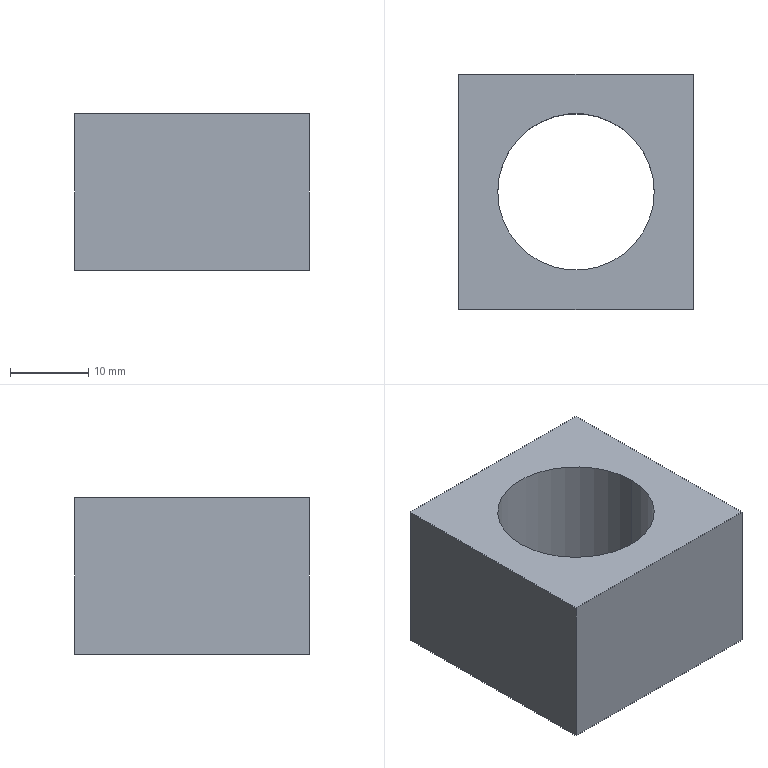Part | SolidWorks | features Extrusion 1 | 1 solid | 8 faces | box 30 x 30 x 20 mm | volume 11717 mm3 | plane 6 | cylinder 2 | commonest cylinder face diameters 20 x2
STEP:
#1=CARTESIAN_POINT('',(-10.,0.,-10.));
#2=VERTEX_POINT('',#1);
#3=CARTESIAN_POINT('',(10.,0.,-10.));
#4=VERTEX_POINT('',#3);
#5=CARTESIAN_POINT('',(0.,0.,-10.));
#6=DIRECTION('',(0.,0.,1.));
#7=DIRECTION('',(-1.,0.,0.));
#8=AXIS2_PLACEMENT_3D('',#5,#6,#7);
#9=CIRCLE('',#8,10.);
#10=EDGE_CURVE('',#2,#4,#9,.T.);
#11=ORIENTED_EDGE('',*,*,#10,.F.);
#12=CARTESIAN_POINT('',(-10.,0.,10.));
#13=VERTEX_POINT('',#12);
#14=CARTESIAN_POINT('',(-10.,0.,-10.));
#15=DIRECTION('',(0.,0.,1.));
#16=VECTOR('',#15,1000.);
#17=LINE('',#14,#16);
#18=EDGE_CURVE('',#2,#13,#17,.T.);
#19=ORIENTED_EDGE('',*,*,#18,.T.);
#20=CARTESIAN_POINT('',(10.,0.,10.));
#21=VERTEX_POINT('',#20);
#22=CARTESIAN_POINT('',(0.,0.,10.));
#23=DIRECTION('',(0.,0.,1.));
#24=DIRECTION('',(-1.,0.,0.));
#25=AXIS2_PLACEMENT_3D('',#22,#23,#24);
#26=CIRCLE('',#25,10.);
#27=EDGE_CURVE('',#13,#21,#26,.T.);
#28=ORIENTED_EDGE('',*,*,#27,.T.);
#29=CARTESIAN_POINT('',(10.,0.,-10.));
#30=DIRECTION('',(0.,0.,1.));
#31=VECTOR('',#30,1000.);
#32=LINE('',#29,#31);
#33=EDGE_CURVE('',#4,#21,#32,.T.);
#34=ORIENTED_EDGE('',*,*,#33,.F.);
#35=EDGE_LOOP('',(#11,#19,#28,#34));
#36=FACE_OUTER_BOUND('',#35,.T.);
#37=CARTESIAN_POINT('',(0.,0.,-10.));
#38=DIRECTION('',(0.,0.,1.));
#39=DIRECTION('',(1.,0.,0.));
#40=AXIS2_PLACEMENT_3D('',#37,#38,#39);
#41=CYLINDRICAL_SURFACE('',#40,10.);
#42=ADVANCED_FACE('',(#36),#41,.F.);
#43=CARTESIAN_POINT('',(-15.,15.,10.));
#44=VERTEX_POINT('',#43);
#45=CARTESIAN_POINT('',(-15.,-15.,10.));
#46=VERTEX_POINT('',#45);
#47=CARTESIAN_POINT('',(-15.,15.,10.));
#48=DIRECTION('',(0.,-1.,0.));
#49=VECTOR('',#48,1000.);
#50=LINE('',#47,#49);
#51=EDGE_CURVE('',#44,#46,#50,.T.);
#52=ORIENTED_EDGE('',*,*,#51,.F.);
#53=CARTESIAN_POINT('',(-15.,15.,-10.));
#54=VERTEX_POINT('',#53);
#55=CARTESIAN_POINT('',(-15.,15.,-10.));
#56=DIRECTION('',(0.,0.,1.));
#57=VECTOR('',#56,1000.);
#58=LINE('',#55,#57);
#59=EDGE_CURVE('',#54,#44,#58,.T.);
#60=ORIENTED_EDGE('',*,*,#59,.F.);
#61=CARTESIAN_POINT('',(-15.,-15.,-10.));
#62=VERTEX_POINT('',#61);
#63=CARTESIAN_POINT('',(-15.,15.,-10.));
#64=DIRECTION('',(0.,-1.,0.));
#65=VECTOR('',#64,1000.);
#66=LINE('',#63,#65);
#67=EDGE_CURVE('',#54,#62,#66,.T.);
#68=ORIENTED_EDGE('',*,*,#67,.T.);
#69=CARTESIAN_POINT('',(-15.,-15.,-10.));
#70=DIRECTION('',(0.,0.,1.));
#71=VECTOR('',#70,1000.);
#72=LINE('',#69,#71);
#73=EDGE_CURVE('',#62,#46,#72,.T.);
#74=ORIENTED_EDGE('',*,*,#73,.T.);
#75=EDGE_LOOP('',(#52,#60,#68,#74));
#76=FACE_OUTER_BOUND('',#75,.T.);
#77=CARTESIAN_POINT('',(-15.,15.,-10.));
#78=DIRECTION('',(-1.,0.,0.));
#79=DIRECTION('',(0.,0.,1.));
#80=AXIS2_PLACEMENT_3D('',#77,#78,#79);
#81=PLANE('',#80);
#82=ADVANCED_FACE('',(#76),#81,.T.);
#83=CARTESIAN_POINT('',(15.,15.,10.));
#84=VERTEX_POINT('',#83);
#85=CARTESIAN_POINT('',(15.,15.,10.));
#86=DIRECTION('',(-1.,0.,0.));
#87=VECTOR('',#86,1000.);
#88=LINE('',#85,#87);
#89=EDGE_CURVE('',#84,#44,#88,.T.);
#90=ORIENTED_EDGE('',*,*,#89,.F.);
#91=CARTESIAN_POINT('',(15.,15.,-10.));
#92=VERTEX_POINT('',#91);
#93=CARTESIAN_POINT('',(15.,15.,-10.));
#94=DIRECTION('',(0.,0.,1.));
#95=VECTOR('',#94,1000.);
#96=LINE('',#93,#95);
#97=EDGE_CURVE('',#92,#84,#96,.T.);
#98=ORIENTED_EDGE('',*,*,#97,.F.);
#99=CARTESIAN_POINT('',(15.,15.,-10.));
#100=DIRECTION('',(-1.,0.,0.));
#101=VECTOR('',#100,1000.);
#102=LINE('',#99,#101);
#103=EDGE_CURVE('',#92,#54,#102,.T.);
#104=ORIENTED_EDGE('',*,*,#103,.T.);
#105=ORIENTED_EDGE('',*,*,#59,.T.);
#106=EDGE_LOOP('',(#90,#98,#104,#105));
#107=FACE_OUTER_BOUND('',#106,.T.);
#108=CARTESIAN_POINT('',(15.,15.,-10.));
#109=DIRECTION('',(0.,1.,0.));
#110=DIRECTION('',(0.,0.,1.));
#111=AXIS2_PLACEMENT_3D('',#108,#109,#110);
#112=PLANE('',#111);
#113=ADVANCED_FACE('',(#107),#112,.T.);
#114=CARTESIAN_POINT('',(15.,-15.,10.));
#115=VERTEX_POINT('',#114);
#116=CARTESIAN_POINT('',(15.,-15.,10.));
#117=DIRECTION('',(0.,1.,0.));
#118=VECTOR('',#117,1000.);
#119=LINE('',#116,#118);
#120=EDGE_CURVE('',#115,#84,#119,.T.);
#121=ORIENTED_EDGE('',*,*,#120,.F.);
#122=CARTESIAN_POINT('',(15.,-15.,-10.));
#123=VERTEX_POINT('',#122);
#124=CARTESIAN_POINT('',(15.,-15.,-10.));
#125=DIRECTION('',(0.,0.,1.));
#126=VECTOR('',#125,1000.);
#127=LINE('',#124,#126);
#128=EDGE_CURVE('',#123,#115,#127,.T.);
#129=ORIENTED_EDGE('',*,*,#128,.F.);
#130=CARTESIAN_POINT('',(15.,-15.,-10.));
#131=DIRECTION('',(0.,1.,0.));
#132=VECTOR('',#131,1000.);
#133=LINE('',#130,#132);
#134=EDGE_CURVE('',#123,#92,#133,.T.);
#135=ORIENTED_EDGE('',*,*,#134,.T.);
#136=ORIENTED_EDGE('',*,*,#97,.T.);
#137=EDGE_LOOP('',(#121,#129,#135,#136));
#138=FACE_OUTER_BOUND('',#137,.T.);
#139=CARTESIAN_POINT('',(15.,-15.,-10.));
#140=DIRECTION('',(1.,0.,0.));
#141=DIRECTION('',(0.,0.,-1.));
#142=AXIS2_PLACEMENT_3D('',#139,#140,#141);
#143=PLANE('',#142);
#144=ADVANCED_FACE('',(#138),#143,.T.);
#145=CARTESIAN_POINT('',(-15.,-15.,10.));
#146=DIRECTION('',(1.,0.,0.));
#147=VECTOR('',#146,1000.);
#148=LINE('',#145,#147);
#149=EDGE_CURVE('',#46,#115,#148,.T.);
#150=ORIENTED_EDGE('',*,*,#149,.F.);
#151=ORIENTED_EDGE('',*,*,#73,.F.);
#152=CARTESIAN_POINT('',(-15.,-15.,-10.));
#153=DIRECTION('',(1.,0.,0.));
#154=VECTOR('',#153,1000.);
#155=LINE('',#152,#154);
#156=EDGE_CURVE('',#62,#123,#155,.T.);
#157=ORIENTED_EDGE('',*,*,#156,.T.);
#158=ORIENTED_EDGE('',*,*,#128,.T.);
#159=EDGE_LOOP('',(#150,#151,#157,#158));
#160=FACE_OUTER_BOUND('',#159,.T.);
#161=CARTESIAN_POINT('',(-15.,-15.,-10.));
#162=DIRECTION('',(0.,-1.,0.));
#163=DIRECTION('',(0.,0.,-1.));
#164=AXIS2_PLACEMENT_3D('',#161,#162,#163);
#165=PLANE('',#164);
#166=ADVANCED_FACE('',(#160),#165,.T.);
#167=CARTESIAN_POINT('',(0.,0.,-10.));
#168=DIRECTION('',(0.,0.,1.));
#169=DIRECTION('',(-1.,0.,0.));
#170=AXIS2_PLACEMENT_3D('',#167,#168,#169);
#171=CIRCLE('',#170,10.);
#172=EDGE_CURVE('',#4,#2,#171,.T.);
#173=ORIENTED_EDGE('',*,*,#172,.T.);
#174=ORIENTED_EDGE('',*,*,#10,.T.);
#175=EDGE_LOOP('',(#173,#174));
#176=FACE_BOUND('',#175,.T.);
#177=ORIENTED_EDGE('',*,*,#67,.F.);
#178=ORIENTED_EDGE('',*,*,#103,.F.);
#179=ORIENTED_EDGE('',*,*,#134,.F.);
#180=ORIENTED_EDGE('',*,*,#156,.F.);
#181=EDGE_LOOP('',(#177,#178,#179,#180));
#182=FACE_OUTER_BOUND('',#181,.T.);
#183=CARTESIAN_POINT('',(0.,0.,-10.));
#184=DIRECTION('',(0.,0.,1.));
#185=DIRECTION('',(1.,0.,0.));
#186=AXIS2_PLACEMENT_3D('',#183,#184,#185);
#187=PLANE('',#186);
#188=ADVANCED_FACE('',(#176,#182),#187,.F.);
#189=CARTESIAN_POINT('',(0.,0.,10.));
#190=DIRECTION('',(0.,0.,1.));
#191=DIRECTION('',(-1.,0.,0.));
#192=AXIS2_PLACEMENT_3D('',#189,#190,#191);
#193=CIRCLE('',#192,10.);
#194=EDGE_CURVE('',#21,#13,#193,.T.);
#195=ORIENTED_EDGE('',*,*,#194,.F.);
#196=ORIENTED_EDGE('',*,*,#27,.F.);
#197=EDGE_LOOP('',(#195,#196));
#198=FACE_BOUND('',#197,.T.);
#199=ORIENTED_EDGE('',*,*,#51,.T.);
#200=ORIENTED_EDGE('',*,*,#149,.T.);
#201=ORIENTED_EDGE('',*,*,#120,.T.);
#202=ORIENTED_EDGE('',*,*,#89,.T.);
#203=EDGE_LOOP('',(#199,#200,#201,#202));
#204=FACE_OUTER_BOUND('',#203,.T.);
#205=CARTESIAN_POINT('',(0.,0.,10.));
#206=DIRECTION('',(0.,0.,1.));
#207=DIRECTION('',(1.,0.,0.));
#208=AXIS2_PLACEMENT_3D('',#205,#206,#207);
#209=PLANE('',#208);
#210=ADVANCED_FACE('',(#198,#204),#209,.T.);
#211=ORIENTED_EDGE('',*,*,#18,.F.);
#212=ORIENTED_EDGE('',*,*,#172,.F.);
#213=ORIENTED_EDGE('',*,*,#33,.T.);
#214=ORIENTED_EDGE('',*,*,#194,.T.);
#215=EDGE_LOOP('',(#211,#212,#213,#214));
#216=FACE_OUTER_BOUND('',#215,.T.);
#217=CARTESIAN_POINT('',(0.,0.,-10.));
#218=DIRECTION('',(0.,0.,1.));
#219=DIRECTION('',(1.,0.,0.));
#220=AXIS2_PLACEMENT_3D('',#217,#218,#219);
#221=CYLINDRICAL_SURFACE('',#220,10.);
#222=ADVANCED_FACE('',(#216),#221,.F.);
#223=CLOSED_SHELL('',(#42,#82,#113,#144,#166,#188,#210,#222));
#224=MANIFOLD_SOLID_BREP('',#223);
#225=CARTESIAN_POINT('',(0.,0.,0.));
#226=DIRECTION('',(0.,0.,1.));
#227=DIRECTION('',(1.,0.,0.));
#228=AXIS2_PLACEMENT_3D('',#225,#226,#227);
#229=(LENGTH_UNIT()NAMED_UNIT(*)SI_UNIT(.MILLI.,.METRE.));
#230=UNCERTAINTY_MEASURE_WITH_UNIT(LENGTH_MEASURE(0.00001),#229,'','');
#231=(NAMED_UNIT(*)PLANE_ANGLE_UNIT()SI_UNIT($,.RADIAN.));
#232=(NAMED_UNIT(*)SI_UNIT($,.STERADIAN.)SOLID_ANGLE_UNIT());
#233=(GEOMETRIC_REPRESENTATION_CONTEXT(3)GLOBAL_UNCERTAINTY_ASSIGNED_CONTEXT((#230))GLOBAL_UNIT_ASSIGNED_CONTEXT((#229,#231,#232))REPRESENTATION_CONTEXT('',''));
#234=ADVANCED_BREP_SHAPE_REPRESENTATION('',(#224,#228),#233);